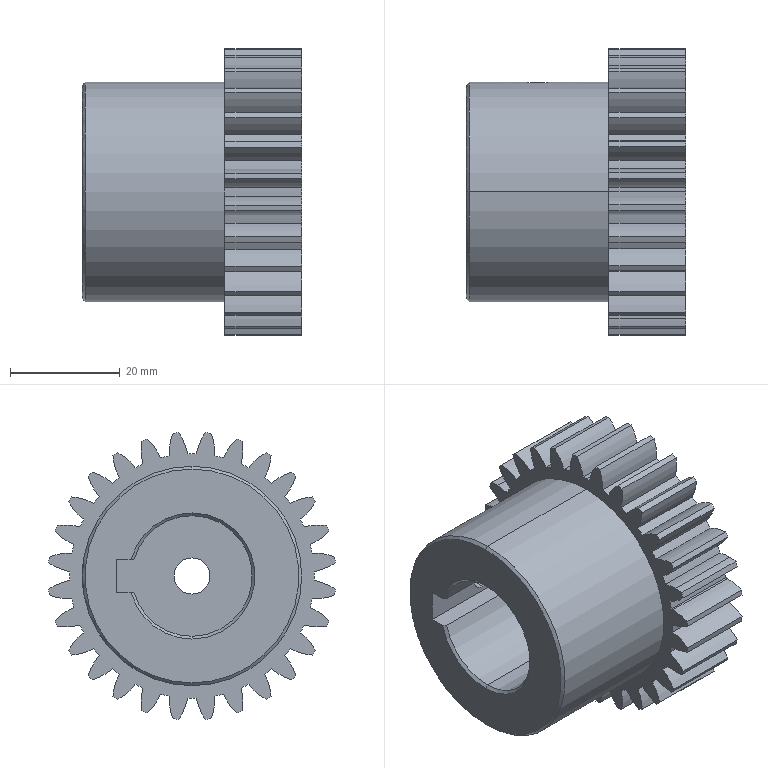Part | 1 solid | 141 faces | box 40 x 52.278 x 52.278 mm | volume 45717 mm3 | cylinder 128 | plane 8 | cone 5 | commonest cylinder face diameters 19.6 x60 44.623 x29 52.5 x28 22 x3 4.2 x2 6.6 x2